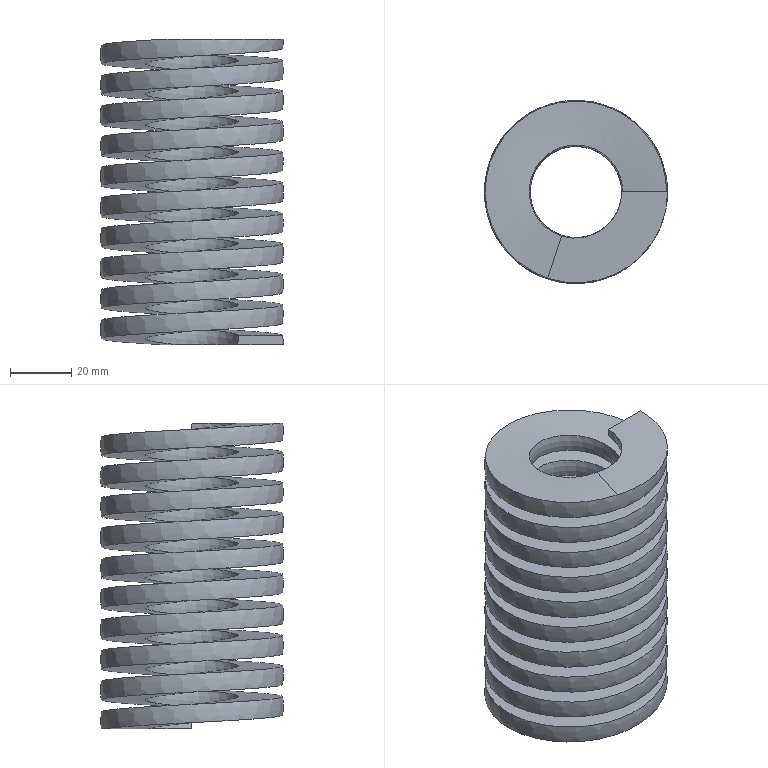Part | Creo | 1 solid | 8 faces | box 60.001 x 60 x 100.003 mm | volume 124605 mm3 | spline 4 | plane 4